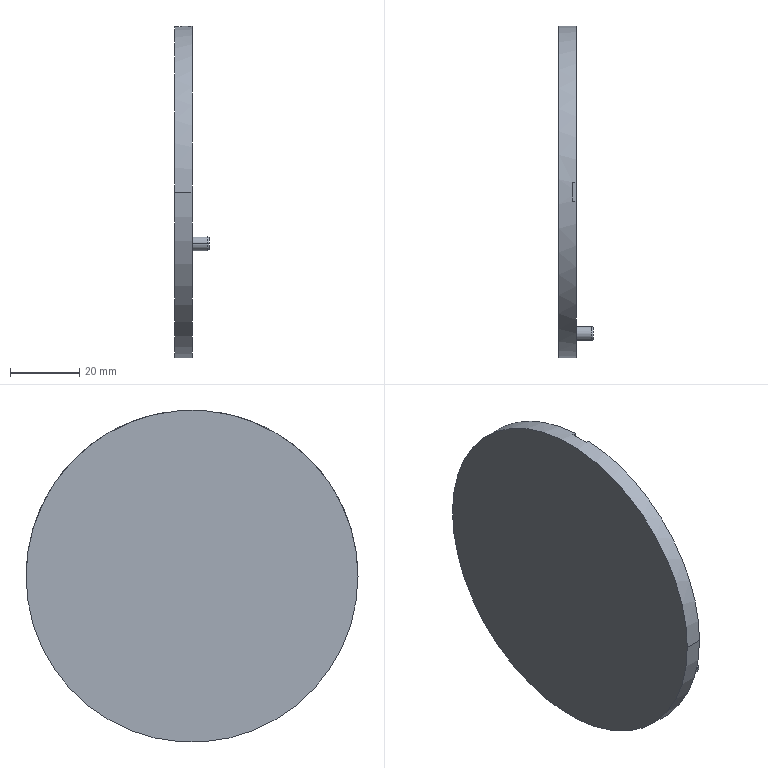Part | STEP file | ASND-0110-IRB120_3-58_IRC5_Link3_rev0 | 2 solids | 14 faces | box 10 x 96 x 96 mm | volume 36166 mm3 | plane 8 | cylinder 4 | cone 2 | commonest cylinder face diameters 4 x2 96 x2
STEP:
#1=CARTESIAN_POINT('',(0.,0.,0.));
#2=DIRECTION('',(0.,0.,1.));
#3=DIRECTION('',(1.,0.,0.));
#4=AXIS2_PLACEMENT_3D('',#1,#2,#3);
#5=CARTESIAN_POINT('',(144.6,48.,630.));
#6=VERTEX_POINT('',#5);
#7=CARTESIAN_POINT('',(144.6,-48.,630.));
#8=VERTEX_POINT('',#7);
#9=CARTESIAN_POINT('',(144.6,0.,630.));
#10=DIRECTION('',(-1.,0.,0.));
#11=DIRECTION('',(0.,1.,0.));
#12=AXIS2_PLACEMENT_3D('',#9,#10,#11);
#13=CIRCLE('',#12,48.);
#14=CARTESIAN_POINT('',(144.6,0.,630.));
#15=DIRECTION('',(1.,0.,0.));
#16=DIRECTION('',(0.,-1.,0.));
#17=AXIS2_PLACEMENT_3D('',#14,#15,#16);
#18=CYLINDRICAL_SURFACE('',#17,48.);
#19=CARTESIAN_POINT('',(3.142,0.));
#20=DIRECTION('',(-1.,0.));
#21=VECTOR('',#20,1.);
#22=LINE('',#19,#21);
#23=(GEOMETRIC_REPRESENTATION_CONTEXT(2)PARAMETRIC_REPRESENTATION_CONTEXT()REPRESENTATION_CONTEXT('',''));
#24=DEFINITIONAL_REPRESENTATION('',(#22),#23);
#25=PCURVE('',#18,#24);
#26=CARTESIAN_POINT('',(144.6,0.,630.));
#27=DIRECTION('',(-1.,0.,0.));
#28=DIRECTION('',(0.,0.7071,0.7071));
#29=AXIS2_PLACEMENT_3D('',#26,#27,#28);
#30=PLANE('',#29);
#31=CARTESIAN_POINT('',(0.,0.));
#32=DIRECTION('',(0.7071,0.7071));
#33=AXIS2_PLACEMENT_2D('',#31,#32);
#34=CIRCLE('',#33,48.);
#35=(GEOMETRIC_REPRESENTATION_CONTEXT(2)PARAMETRIC_REPRESENTATION_CONTEXT()REPRESENTATION_CONTEXT('',''));
#36=DEFINITIONAL_REPRESENTATION('',(#34),#35);
#37=PCURVE('',#30,#36);
#38=SURFACE_CURVE('',#13,(#25,#37),.PCURVE_S1.);
#39=EDGE_CURVE('',#6,#8,#38,.T.);
#40=ORIENTED_EDGE('',*,*,#39,.F.);
#41=CARTESIAN_POINT('',(149.6,48.,630.));
#42=VERTEX_POINT('',#41);
#43=CARTESIAN_POINT('',(144.6,48.,630.));
#44=DIRECTION('',(1.,0.,0.));
#45=VECTOR('',#44,1.);
#46=LINE('',#43,#45);
#47=CARTESIAN_POINT('',(3.142,0.));
#48=DIRECTION('',(0.,1.));
#49=VECTOR('',#48,1.);
#50=LINE('',#47,#49);
#51=(GEOMETRIC_REPRESENTATION_CONTEXT(2)PARAMETRIC_REPRESENTATION_CONTEXT()REPRESENTATION_CONTEXT('',''));
#52=DEFINITIONAL_REPRESENTATION('',(#50),#51);
#53=PCURVE('',#18,#52);
#54=CARTESIAN_POINT('',(144.6,0.,630.));
#55=DIRECTION('',(1.,0.,0.));
#56=DIRECTION('',(0.,-1.,0.));
#57=AXIS2_PLACEMENT_3D('',#54,#55,#56);
#58=CYLINDRICAL_SURFACE('',#57,48.);
#59=CARTESIAN_POINT('',(3.142,0.));
#60=DIRECTION('',(0.,1.));
#61=VECTOR('',#60,1.);
#62=LINE('',#59,#61);
#63=(GEOMETRIC_REPRESENTATION_CONTEXT(2)PARAMETRIC_REPRESENTATION_CONTEXT()REPRESENTATION_CONTEXT('',''));
#64=DEFINITIONAL_REPRESENTATION('',(#62),#63);
#65=PCURVE('',#58,#64);
#66=SURFACE_CURVE('',#46,(#53,#65),.PCURVE_S1.);
#67=EDGE_CURVE('',#6,#42,#66,.T.);
#68=ORIENTED_EDGE('',*,*,#67,.T.);
#69=CARTESIAN_POINT('',(149.6,-48.,630.));
#70=VERTEX_POINT('',#69);
#71=CARTESIAN_POINT('',(149.6,0.,630.));
#72=DIRECTION('',(-1.,0.,0.));
#73=DIRECTION('',(0.,1.,0.));
#74=AXIS2_PLACEMENT_3D('',#71,#72,#73);
#75=CIRCLE('',#74,48.);
#76=CARTESIAN_POINT('',(3.142,5.));
#77=DIRECTION('',(-1.,0.));
#78=VECTOR('',#77,1.);
#79=LINE('',#76,#78);
#80=(GEOMETRIC_REPRESENTATION_CONTEXT(2)PARAMETRIC_REPRESENTATION_CONTEXT()REPRESENTATION_CONTEXT('',''));
#81=DEFINITIONAL_REPRESENTATION('',(#79),#80);
#82=PCURVE('',#18,#81);
#83=CARTESIAN_POINT('',(149.6,0.,630.));
#84=DIRECTION('',(-1.,0.,0.));
#85=DIRECTION('',(0.,0.7071,0.7071));
#86=AXIS2_PLACEMENT_3D('',#83,#84,#85);
#87=PLANE('',#86);
#88=CARTESIAN_POINT('',(0.,0.));
#89=DIRECTION('',(0.7071,0.7071));
#90=AXIS2_PLACEMENT_2D('',#88,#89);
#91=CIRCLE('',#90,48.);
#92=(GEOMETRIC_REPRESENTATION_CONTEXT(2)PARAMETRIC_REPRESENTATION_CONTEXT()REPRESENTATION_CONTEXT('',''));
#93=DEFINITIONAL_REPRESENTATION('',(#91),#92);
#94=PCURVE('',#87,#93);
#95=SURFACE_CURVE('',#75,(#82,#94),.PCURVE_S1.);
#96=EDGE_CURVE('',#42,#70,#95,.T.);
#97=ORIENTED_EDGE('',*,*,#96,.T.);
#98=CARTESIAN_POINT('',(144.6,-48.,630.));
#99=DIRECTION('',(1.,0.,0.));
#100=VECTOR('',#99,1.);
#101=LINE('',#98,#100);
#102=CARTESIAN_POINT('',(0.,0.));
#103=DIRECTION('',(0.,1.));
#104=VECTOR('',#103,1.);
#105=LINE('',#102,#104);
#106=(GEOMETRIC_REPRESENTATION_CONTEXT(2)PARAMETRIC_REPRESENTATION_CONTEXT()REPRESENTATION_CONTEXT('',''));
#107=DEFINITIONAL_REPRESENTATION('',(#105),#106);
#108=PCURVE('',#18,#107);
#109=CARTESIAN_POINT('',(6.283,0.));
#110=DIRECTION('',(0.,1.));
#111=VECTOR('',#110,1.);
#112=LINE('',#109,#111);
#113=(GEOMETRIC_REPRESENTATION_CONTEXT(2)PARAMETRIC_REPRESENTATION_CONTEXT()REPRESENTATION_CONTEXT('',''));
#114=DEFINITIONAL_REPRESENTATION('',(#112),#113);
#115=PCURVE('',#58,#114);
#116=SURFACE_CURVE('',#101,(#108,#115),.PCURVE_S1.);
#117=EDGE_CURVE('',#8,#70,#116,.T.);
#118=ORIENTED_EDGE('',*,*,#117,.F.);
#119=EDGE_LOOP('',(#40,#68,#97,#118));
#120=FACE_BOUND('',#119,.T.);
#121=ADVANCED_FACE('',(#120),#18,.T.);
#122=ORIENTED_EDGE('',*,*,#67,.F.);
#123=CARTESIAN_POINT('',(144.6,0.,630.));
#124=DIRECTION('',(-1.,0.,0.));
#125=DIRECTION('',(0.,1.,0.));
#126=AXIS2_PLACEMENT_3D('',#123,#124,#125);
#127=CIRCLE('',#126,48.);
#128=CARTESIAN_POINT('',(9.425,0.));
#129=DIRECTION('',(-1.,0.));
#130=VECTOR('',#129,1.);
#131=LINE('',#128,#130);
#132=(GEOMETRIC_REPRESENTATION_CONTEXT(2)PARAMETRIC_REPRESENTATION_CONTEXT()REPRESENTATION_CONTEXT('',''));
#133=DEFINITIONAL_REPRESENTATION('',(#131),#132);
#134=PCURVE('',#58,#133);
#135=CARTESIAN_POINT('',(0.,0.));
#136=DIRECTION('',(0.7071,0.7071));
#137=AXIS2_PLACEMENT_2D('',#135,#136);
#138=CIRCLE('',#137,48.);
#139=(GEOMETRIC_REPRESENTATION_CONTEXT(2)PARAMETRIC_REPRESENTATION_CONTEXT()REPRESENTATION_CONTEXT('',''));
#140=DEFINITIONAL_REPRESENTATION('',(#138),#139);
#141=PCURVE('',#30,#140);
#142=SURFACE_CURVE('',#127,(#134,#141),.PCURVE_S1.);
#143=EDGE_CURVE('',#8,#6,#142,.T.);
#144=ORIENTED_EDGE('',*,*,#143,.F.);
#145=ORIENTED_EDGE('',*,*,#117,.T.);
#146=CARTESIAN_POINT('',(149.6,-2.75,677.921));
#147=VERTEX_POINT('',#146);
#148=CARTESIAN_POINT('',(149.6,0.,630.));
#149=DIRECTION('',(-1.,0.,0.));
#150=DIRECTION('',(0.,1.,0.));
#151=AXIS2_PLACEMENT_3D('',#148,#149,#150);
#152=CIRCLE('',#151,48.);
#153=CARTESIAN_POINT('',(9.425,5.));
#154=DIRECTION('',(-1.,0.));
#155=VECTOR('',#154,1.);
#156=LINE('',#153,#155);
#157=(GEOMETRIC_REPRESENTATION_CONTEXT(2)PARAMETRIC_REPRESENTATION_CONTEXT()REPRESENTATION_CONTEXT('',''));
#158=DEFINITIONAL_REPRESENTATION('',(#156),#157);
#159=PCURVE('',#58,#158);
#160=CARTESIAN_POINT('',(0.,0.));
#161=DIRECTION('',(0.7071,0.7071));
#162=AXIS2_PLACEMENT_2D('',#160,#161);
#163=CIRCLE('',#162,48.);
#164=(GEOMETRIC_REPRESENTATION_CONTEXT(2)PARAMETRIC_REPRESENTATION_CONTEXT()REPRESENTATION_CONTEXT('',''));
#165=DEFINITIONAL_REPRESENTATION('',(#163),#164);
#166=PCURVE('',#87,#165);
#167=SURFACE_CURVE('',#152,(#159,#166),.PCURVE_S1.);
#168=EDGE_CURVE('',#70,#147,#167,.T.);
#169=ORIENTED_EDGE('',*,*,#168,.T.);
#170=CARTESIAN_POINT('',(148.6,-2.75,677.921));
#171=VERTEX_POINT('',#170);
#172=CARTESIAN_POINT('',(148.6,-2.75,677.921));
#173=DIRECTION('',(-1.,0.,0.));
#174=VECTOR('',#173,1.);
#175=LINE('',#172,#174);
#176=CARTESIAN_POINT('',(4.77,4.));
#177=DIRECTION('',(0.,-1.));
#178=VECTOR('',#177,1.);
#179=LINE('',#176,#178);
#180=(GEOMETRIC_REPRESENTATION_CONTEXT(2)PARAMETRIC_REPRESENTATION_CONTEXT()REPRESENTATION_CONTEXT('',''));
#181=DEFINITIONAL_REPRESENTATION('',(#179),#180);
#182=PCURVE('',#58,#181);
#183=CARTESIAN_POINT('',(148.6,-2.75,662.));
#184=DIRECTION('',(0.,-1.,0.));
#185=DIRECTION('',(0.7071,0.,0.7071));
#186=AXIS2_PLACEMENT_3D('',#183,#184,#185);
#187=PLANE('',#186);
#188=CARTESIAN_POINT('',(11.258,11.258));
#189=DIRECTION('',(-0.7071,0.7071));
#190=VECTOR('',#189,1.);
#191=LINE('',#188,#190);
#192=(GEOMETRIC_REPRESENTATION_CONTEXT(2)PARAMETRIC_REPRESENTATION_CONTEXT()REPRESENTATION_CONTEXT('',''));
#193=DEFINITIONAL_REPRESENTATION('',(#191),#192);
#194=PCURVE('',#187,#193);
#195=SURFACE_CURVE('',#175,(#182,#194),.PCURVE_S1.);
#196=EDGE_CURVE('',#147,#171,#195,.T.);
#197=ORIENTED_EDGE('',*,*,#196,.T.);
#198=CARTESIAN_POINT('',(148.6,2.75,677.921));
#199=VERTEX_POINT('',#198);
#200=CARTESIAN_POINT('',(148.6,0.,630.));
#201=DIRECTION('',(1.,0.,0.));
#202=DIRECTION('',(0.,-1.,0.));
#203=AXIS2_PLACEMENT_3D('',#200,#201,#202);
#204=CIRCLE('',#203,48.);
#205=CARTESIAN_POINT('',(0.,4.));
#206=DIRECTION('',(1.,0.));
#207=VECTOR('',#206,1.);
#208=LINE('',#205,#207);
#209=(GEOMETRIC_REPRESENTATION_CONTEXT(2)PARAMETRIC_REPRESENTATION_CONTEXT()REPRESENTATION_CONTEXT('',''));
#210=DEFINITIONAL_REPRESENTATION('',(#208),#209);
#211=PCURVE('',#58,#210);
#212=CARTESIAN_POINT('',(148.6,2.75,682.));
#213=DIRECTION('',(1.,0.,0.));
#214=DIRECTION('',(0.,0.7071,0.7071));
#215=AXIS2_PLACEMENT_3D('',#212,#213,#214);
#216=PLANE('',#215);
#217=CARTESIAN_POINT('',(-38.714,-34.825));
#218=DIRECTION('',(-0.7071,0.7071));
#219=AXIS2_PLACEMENT_2D('',#217,#218);
#220=CIRCLE('',#219,48.);
#221=(GEOMETRIC_REPRESENTATION_CONTEXT(2)PARAMETRIC_REPRESENTATION_CONTEXT()REPRESENTATION_CONTEXT('',''));
#222=DEFINITIONAL_REPRESENTATION('',(#220),#221);
#223=PCURVE('',#216,#222);
#224=SURFACE_CURVE('',#204,(#211,#223),.PCURVE_S1.);
#225=EDGE_CURVE('',#199,#171,#224,.T.);
#226=ORIENTED_EDGE('',*,*,#225,.F.);
#227=CARTESIAN_POINT('',(149.6,2.75,677.921));
#228=VERTEX_POINT('',#227);
#229=CARTESIAN_POINT('',(148.6,2.75,677.921));
#230=DIRECTION('',(1.,0.,0.));
#231=VECTOR('',#230,1.);
#232=LINE('',#229,#231);
#233=CARTESIAN_POINT('',(4.655,4.));
#234=DIRECTION('',(0.,1.));
#235=VECTOR('',#234,1.);
#236=LINE('',#233,#235);
#237=(GEOMETRIC_REPRESENTATION_CONTEXT(2)PARAMETRIC_REPRESENTATION_CONTEXT()REPRESENTATION_CONTEXT('',''));
#238=DEFINITIONAL_REPRESENTATION('',(#236),#237);
#239=PCURVE('',#58,#238);
#240=CARTESIAN_POINT('',(148.6,2.75,662.));
#241=DIRECTION('',(0.,1.,0.));
#242=DIRECTION('',(0.7071,0.,0.7071));
#243=AXIS2_PLACEMENT_3D('',#240,#241,#242);
#244=PLANE('',#243);
#245=CARTESIAN_POINT('',(11.258,-11.258));
#246=DIRECTION('',(0.7071,0.7071));
#247=VECTOR('',#246,1.);
#248=LINE('',#245,#247);
#249=(GEOMETRIC_REPRESENTATION_CONTEXT(2)PARAMETRIC_REPRESENTATION_CONTEXT()REPRESENTATION_CONTEXT('',''));
#250=DEFINITIONAL_REPRESENTATION('',(#248),#249);
#251=PCURVE('',#244,#250);
#252=SURFACE_CURVE('',#232,(#239,#251),.PCURVE_S1.);
#253=EDGE_CURVE('',#199,#228,#252,.T.);
#254=ORIENTED_EDGE('',*,*,#253,.T.);
#255=CARTESIAN_POINT('',(149.6,0.,630.));
#256=DIRECTION('',(-1.,0.,0.));
#257=DIRECTION('',(0.,1.,0.));
#258=AXIS2_PLACEMENT_3D('',#255,#256,#257);
#259=CIRCLE('',#258,48.);
#260=CARTESIAN_POINT('',(9.425,5.));
#261=DIRECTION('',(-1.,0.));
#262=VECTOR('',#261,1.);
#263=LINE('',#260,#262);
#264=(GEOMETRIC_REPRESENTATION_CONTEXT(2)PARAMETRIC_REPRESENTATION_CONTEXT()REPRESENTATION_CONTEXT('',''));
#265=DEFINITIONAL_REPRESENTATION('',(#263),#264);
#266=PCURVE('',#58,#265);
#267=CARTESIAN_POINT('',(0.,0.));
#268=DIRECTION('',(0.7071,0.7071));
#269=AXIS2_PLACEMENT_2D('',#267,#268);
#270=CIRCLE('',#269,48.);
#271=(GEOMETRIC_REPRESENTATION_CONTEXT(2)PARAMETRIC_REPRESENTATION_CONTEXT()REPRESENTATION_CONTEXT('',''));
#272=DEFINITIONAL_REPRESENTATION('',(#270),#271);
#273=PCURVE('',#87,#272);
#274=SURFACE_CURVE('',#259,(#266,#273),.PCURVE_S1.);
#275=EDGE_CURVE('',#228,#42,#274,.T.);
#276=ORIENTED_EDGE('',*,*,#275,.T.);
#277=EDGE_LOOP('',(#122,#144,#145,#169,#197,#226,#254,#276));
#278=FACE_BOUND('',#277,.T.);
#279=ADVANCED_FACE('',(#278),#58,.T.);
#280=ORIENTED_EDGE('',*,*,#143,.T.);
#281=ORIENTED_EDGE('',*,*,#39,.T.);
#282=EDGE_LOOP('',(#280,#281));
#283=FACE_BOUND('',#282,.T.);
#284=ADVANCED_FACE('',(#283),#30,.T.);
#285=ORIENTED_EDGE('',*,*,#275,.F.);
#286=CARTESIAN_POINT('',(149.6,2.75,662.));
#287=VERTEX_POINT('',#286);
#288=CARTESIAN_POINT('',(149.6,2.75,662.));
#289=DIRECTION('',(0.,0.,1.));
#290=VECTOR('',#289,1.);
#291=LINE('',#288,#290);
#292=CARTESIAN_POINT('',(24.572,-20.683));
#293=DIRECTION('',(0.7071,-0.7071));
#294=VECTOR('',#293,1.);
#295=LINE('',#292,#294);
#296=(GEOMETRIC_REPRESENTATION_CONTEXT(2)PARAMETRIC_REPRESENTATION_CONTEXT()REPRESENTATION_CONTEXT('',''));
#297=DEFINITIONAL_REPRESENTATION('',(#295),#296);
#298=PCURVE('',#87,#297);
#299=CARTESIAN_POINT('',(0.7071,0.7071));
#300=DIRECTION('',(0.7071,-0.7071));
#301=VECTOR('',#300,1.);
#302=LINE('',#299,#301);
#303=(GEOMETRIC_REPRESENTATION_CONTEXT(2)PARAMETRIC_REPRESENTATION_CONTEXT()REPRESENTATION_CONTEXT('',''));
#304=DEFINITIONAL_REPRESENTATION('',(#302),#303);
#305=PCURVE('',#244,#304);
#306=SURFACE_CURVE('',#291,(#298,#305),.PCURVE_S1.);
#307=EDGE_CURVE('',#287,#228,#306,.T.);
#308=ORIENTED_EDGE('',*,*,#307,.F.);
#309=CARTESIAN_POINT('',(149.6,-2.75,662.));
#310=VERTEX_POINT('',#309);
#311=CARTESIAN_POINT('',(149.6,-2.75,662.));
#312=DIRECTION('',(0.,1.,0.));
#313=VECTOR('',#312,1.);
#314=LINE('',#311,#313);
#315=CARTESIAN_POINT('',(20.683,-24.572));
#316=DIRECTION('',(0.7071,0.7071));
#317=VECTOR('',#316,1.);
#318=LINE('',#315,#317);
#319=(GEOMETRIC_REPRESENTATION_CONTEXT(2)PARAMETRIC_REPRESENTATION_CONTEXT()REPRESENTATION_CONTEXT('',''));
#320=DEFINITIONAL_REPRESENTATION('',(#318),#319);
#321=PCURVE('',#87,#320);
#322=CARTESIAN_POINT('',(148.6,2.75,662.));
#323=DIRECTION('',(0.,0.,-1.));
#324=DIRECTION('',(0.7071,0.7071,0.));
#325=AXIS2_PLACEMENT_3D('',#322,#323,#324);
#326=PLANE('',#325);
#327=CARTESIAN_POINT('',(-3.182,4.596));
#328=DIRECTION('',(0.7071,-0.7071));
#329=VECTOR('',#328,1.);
#330=LINE('',#327,#329);
#331=(GEOMETRIC_REPRESENTATION_CONTEXT(2)PARAMETRIC_REPRESENTATION_CONTEXT()REPRESENTATION_CONTEXT('',''));
#332=DEFINITIONAL_REPRESENTATION('',(#330),#331);
#333=PCURVE('',#326,#332);
#334=SURFACE_CURVE('',#314,(#321,#333),.PCURVE_S1.);
#335=EDGE_CURVE('',#310,#287,#334,.T.);
#336=ORIENTED_EDGE('',*,*,#335,.F.);
#337=CARTESIAN_POINT('',(149.6,-2.75,662.));
#338=DIRECTION('',(0.,0.,1.));
#339=VECTOR('',#338,1.);
#340=LINE('',#337,#339);
#341=CARTESIAN_POINT('',(20.683,-24.572));
#342=DIRECTION('',(0.7071,-0.7071));
#343=VECTOR('',#342,1.);
#344=LINE('',#341,#343);
#345=(GEOMETRIC_REPRESENTATION_CONTEXT(2)PARAMETRIC_REPRESENTATION_CONTEXT()REPRESENTATION_CONTEXT('',''));
#346=DEFINITIONAL_REPRESENTATION('',(#344),#345);
#347=PCURVE('',#87,#346);
#348=CARTESIAN_POINT('',(0.7071,-0.7071));
#349=DIRECTION('',(0.7071,0.7071));
#350=VECTOR('',#349,1.);
#351=LINE('',#348,#350);
#352=(GEOMETRIC_REPRESENTATION_CONTEXT(2)PARAMETRIC_REPRESENTATION_CONTEXT()REPRESENTATION_CONTEXT('',''));
#353=DEFINITIONAL_REPRESENTATION('',(#351),#352);
#354=PCURVE('',#187,#353);
#355=SURFACE_CURVE('',#340,(#347,#354),.PCURVE_S1.);
#356=EDGE_CURVE('',#310,#147,#355,.T.);
#357=ORIENTED_EDGE('',*,*,#356,.T.);
#358=ORIENTED_EDGE('',*,*,#168,.F.);
#359=ORIENTED_EDGE('',*,*,#96,.F.);
#360=EDGE_LOOP('',(#285,#308,#336,#357,#358,#359));
#361=FACE_BOUND('',#360,.T.);
#362=ADVANCED_FACE('',(#361),#87,.F.);
#363=ORIENTED_EDGE('',*,*,#225,.T.);
#364=CARTESIAN_POINT('',(148.6,-2.75,662.));
#365=VERTEX_POINT('',#364);
#366=CARTESIAN_POINT('',(148.6,-2.75,677.921));
#367=DIRECTION('',(0.,0.,-1.));
#368=VECTOR('',#367,1.);
#369=LINE('',#366,#368);
#370=CARTESIAN_POINT('',(-6.773,1.005));
#371=DIRECTION('',(-0.7071,-0.7071));
#372=VECTOR('',#371,1.);
#373=LINE('',#370,#372);
#374=(GEOMETRIC_REPRESENTATION_CONTEXT(2)PARAMETRIC_REPRESENTATION_CONTEXT()REPRESENTATION_CONTEXT('',''));
#375=DEFINITIONAL_REPRESENTATION('',(#373),#374);
#376=PCURVE('',#216,#375);
#377=CARTESIAN_POINT('',(11.258,11.258));
#378=DIRECTION('',(-0.7071,-0.7071));
#379=VECTOR('',#378,1.);
#380=LINE('',#377,#379);
#381=(GEOMETRIC_REPRESENTATION_CONTEXT(2)PARAMETRIC_REPRESENTATION_CONTEXT()REPRESENTATION_CONTEXT('',''));
#382=DEFINITIONAL_REPRESENTATION('',(#380),#381);
#383=PCURVE('',#187,#382);
#384=SURFACE_CURVE('',#369,(#376,#383),.PCURVE_S1.);
#385=EDGE_CURVE('',#171,#365,#384,.T.);
#386=ORIENTED_EDGE('',*,*,#385,.T.);
#387=CARTESIAN_POINT('',(148.6,2.75,662.));
#388=VERTEX_POINT('',#387);
#389=CARTESIAN_POINT('',(148.6,-2.75,662.));
#390=DIRECTION('',(0.,1.,0.));
#391=VECTOR('',#390,1.);
#392=LINE('',#389,#391);
#393=CARTESIAN_POINT('',(-18.031,-10.253));
#394=DIRECTION('',(0.7071,-0.7071));
#395=VECTOR('',#394,1.);
#396=LINE('',#393,#395);
#397=(GEOMETRIC_REPRESENTATION_CONTEXT(2)PARAMETRIC_REPRESENTATION_CONTEXT()REPRESENTATION_CONTEXT('',''));
#398=DEFINITIONAL_REPRESENTATION('',(#396),#397);
#399=PCURVE('',#216,#398);
#400=CARTESIAN_POINT('',(-3.889,3.889));
#401=DIRECTION('',(0.7071,-0.7071));
#402=VECTOR('',#401,1.);
#403=LINE('',#400,#402);
#404=(GEOMETRIC_REPRESENTATION_CONTEXT(2)PARAMETRIC_REPRESENTATION_CONTEXT()REPRESENTATION_CONTEXT('',''));
#405=DEFINITIONAL_REPRESENTATION('',(#403),#404);
#406=PCURVE('',#326,#405);
#407=SURFACE_CURVE('',#392,(#399,#406),.PCURVE_S1.);
#408=EDGE_CURVE('',#365,#388,#407,.T.);
#409=ORIENTED_EDGE('',*,*,#408,.T.);
#410=CARTESIAN_POINT('',(148.6,2.75,662.));
#411=DIRECTION('',(0.,0.,1.));
#412=VECTOR('',#411,1.);
#413=LINE('',#410,#412);
#414=CARTESIAN_POINT('',(-14.142,-14.142));
#415=DIRECTION('',(0.7071,0.7071));
#416=VECTOR('',#415,1.);
#417=LINE('',#414,#416);
#418=(GEOMETRIC_REPRESENTATION_CONTEXT(2)PARAMETRIC_REPRESENTATION_CONTEXT()REPRESENTATION_CONTEXT('',''));
#419=DEFINITIONAL_REPRESENTATION('',(#417),#418);
#420=PCURVE('',#216,#419);
#421=CARTESIAN_POINT('',(0.,0.));
#422=DIRECTION('',(0.7071,-0.7071));
#423=VECTOR('',#422,1.);
#424=LINE('',#421,#423);
#425=(GEOMETRIC_REPRESENTATION_CONTEXT(2)PARAMETRIC_REPRESENTATION_CONTEXT()REPRESENTATION_CONTEXT('',''));
#426=DEFINITIONAL_REPRESENTATION('',(#424),#425);
#427=PCURVE('',#244,#426);
#428=SURFACE_CURVE('',#413,(#420,#427),.PCURVE_S1.);
#429=EDGE_CURVE('',#388,#199,#428,.T.);
#430=ORIENTED_EDGE('',*,*,#429,.T.);
#431=EDGE_LOOP('',(#363,#386,#409,#430));
#432=FACE_BOUND('',#431,.T.);
#433=ADVANCED_FACE('',(#432),#216,.T.);
#434=ORIENTED_EDGE('',*,*,#429,.F.);
#435=CARTESIAN_POINT('',(148.6,2.75,662.));
#436=DIRECTION('',(1.,0.,0.));
#437=VECTOR('',#436,1.);
#438=LINE('',#435,#437);
#439=CARTESIAN_POINT('',(0.,0.));
#440=DIRECTION('',(0.7071,0.7071));
#441=VECTOR('',#440,1.);
#442=LINE('',#439,#441);
#443=(GEOMETRIC_REPRESENTATION_CONTEXT(2)PARAMETRIC_REPRESENTATION_CONTEXT()REPRESENTATION_CONTEXT('',''));
#444=DEFINITIONAL_REPRESENTATION('',(#442),#443);
#445=PCURVE('',#244,#444);
#446=CARTESIAN_POINT('',(0.,0.));
#447=DIRECTION('',(0.7071,0.7071));
#448=VECTOR('',#447,1.);
#449=LINE('',#446,#448);
#450=(GEOMETRIC_REPRESENTATION_CONTEXT(2)PARAMETRIC_REPRESENTATION_CONTEXT()REPRESENTATION_CONTEXT('',''));
#451=DEFINITIONAL_REPRESENTATION('',(#449),#450);
#452=PCURVE('',#326,#451);
#453=SURFACE_CURVE('',#438,(#445,#452),.PCURVE_S1.);
#454=EDGE_CURVE('',#388,#287,#453,.T.);
#455=ORIENTED_EDGE('',*,*,#454,.T.);
#456=ORIENTED_EDGE('',*,*,#307,.T.);
#457=ORIENTED_EDGE('',*,*,#253,.F.);
#458=EDGE_LOOP('',(#434,#455,#456,#457));
#459=FACE_BOUND('',#458,.T.);
#460=ADVANCED_FACE('',(#459),#244,.F.);
#461=ORIENTED_EDGE('',*,*,#356,.F.);
#462=CARTESIAN_POINT('',(148.6,-2.75,662.));
#463=DIRECTION('',(1.,0.,0.));
#464=VECTOR('',#463,1.);
#465=LINE('',#462,#464);
#466=CARTESIAN_POINT('',(0.,0.));
#467=DIRECTION('',(0.7071,-0.7071));
#468=VECTOR('',#467,1.);
#469=LINE('',#466,#468);
#470=(GEOMETRIC_REPRESENTATION_CONTEXT(2)PARAMETRIC_REPRESENTATION_CONTEXT()REPRESENTATION_CONTEXT('',''));
#471=DEFINITIONAL_REPRESENTATION('',(#469),#470);
#472=PCURVE('',#187,#471);
#473=CARTESIAN_POINT('',(-3.889,3.889));
#474=DIRECTION('',(0.7071,0.7071));
#475=VECTOR('',#474,1.);
#476=LINE('',#473,#475);
#477=(GEOMETRIC_REPRESENTATION_CONTEXT(2)PARAMETRIC_REPRESENTATION_CONTEXT()REPRESENTATION_CONTEXT('',''));
#478=DEFINITIONAL_REPRESENTATION('',(#476),#477);
#479=PCURVE('',#326,#478);
#480=SURFACE_CURVE('',#465,(#472,#479),.PCURVE_S1.);
#481=EDGE_CURVE('',#365,#310,#480,.T.);
#482=ORIENTED_EDGE('',*,*,#481,.F.);
#483=ORIENTED_EDGE('',*,*,#385,.F.);
#484=ORIENTED_EDGE('',*,*,#196,.F.);
#485=EDGE_LOOP('',(#461,#482,#483,#484));
#486=FACE_BOUND('',#485,.T.);
#487=ADVANCED_FACE('',(#486),#187,.F.);
#488=ORIENTED_EDGE('',*,*,#335,.T.);
#489=ORIENTED_EDGE('',*,*,#454,.F.);
#490=ORIENTED_EDGE('',*,*,#408,.F.);
#491=ORIENTED_EDGE('',*,*,#481,.T.);
#492=EDGE_LOOP('',(#488,#489,#490,#491));
#493=FACE_BOUND('',#492,.T.);
#494=ADVANCED_FACE('',(#493),#326,.F.);
#495=CLOSED_SHELL('',(#121,#279,#284,#362,#433,#460,#487,#494));
#496=MANIFOLD_SOLID_BREP('',#495);
#497=CARTESIAN_POINT('',(154.6,-42.716,615.122));
#498=VERTEX_POINT('',#497);
#499=CARTESIAN_POINT('',(154.6,-39.037,615.122));
#500=VERTEX_POINT('',#499);
#501=CARTESIAN_POINT('',(154.6,-40.877,615.122));
#502=DIRECTION('',(-1.,0.,0.));
#503=DIRECTION('',(0.,-1.,0.));
#504=AXIS2_PLACEMENT_3D('',#501,#502,#503);
#505=CIRCLE('',#504,1.839);
#506=CARTESIAN_POINT('',(154.6,-40.877,615.122));
#507=DIRECTION('',(-1.,0.,0.));
#508=DIRECTION('',(0.,-1.,0.));
#509=AXIS2_PLACEMENT_3D('',#506,#507,#508);
#510=CONICAL_SURFACE('',#509,1.839,0.2618);
#511=CARTESIAN_POINT('',(0.,0.));
#512=DIRECTION('',(1.,0.));
#513=VECTOR('',#512,1.);
#514=LINE('',#511,#513);
#515=(GEOMETRIC_REPRESENTATION_CONTEXT(2)PARAMETRIC_REPRESENTATION_CONTEXT()REPRESENTATION_CONTEXT('',''));
#516=DEFINITIONAL_REPRESENTATION('',(#514),#515);
#517=PCURVE('',#510,#516);
#518=CARTESIAN_POINT('',(154.6,-39.037,615.122));
#519=DIRECTION('',(-1.,0.,0.));
#520=DIRECTION('',(0.,0.7071,0.7071));
#521=AXIS2_PLACEMENT_3D('',#518,#519,#520);
#522=PLANE('',#521);
#523=CARTESIAN_POINT('',(-1.301,-1.301));
#524=DIRECTION('',(-0.7071,-0.7071));
#525=AXIS2_PLACEMENT_2D('',#523,#524);
#526=CIRCLE('',#525,1.839);
#527=(GEOMETRIC_REPRESENTATION_CONTEXT(2)PARAMETRIC_REPRESENTATION_CONTEXT()REPRESENTATION_CONTEXT('',''));
#528=DEFINITIONAL_REPRESENTATION('',(#526),#527);
#529=PCURVE('',#522,#528);
#530=SURFACE_CURVE('',#505,(#517,#529),.PCURVE_S1.);
#531=EDGE_CURVE('',#498,#500,#530,.T.);
#532=ORIENTED_EDGE('',*,*,#531,.T.);
#533=CARTESIAN_POINT('',(154.,-38.877,615.122));
#534=VERTEX_POINT('',#533);
#535=CARTESIAN_POINT('',(154.6,-39.037,615.122));
#536=DIRECTION('',(-0.9659,0.2588,0.));
#537=VECTOR('',#536,1.);
#538=LINE('',#535,#537);
#539=CARTESIAN_POINT('',(3.142,0.));
#540=DIRECTION('',(0.,1.));
#541=VECTOR('',#540,1.);
#542=LINE('',#539,#541);
#543=(GEOMETRIC_REPRESENTATION_CONTEXT(2)PARAMETRIC_REPRESENTATION_CONTEXT()REPRESENTATION_CONTEXT('',''));
#544=DEFINITIONAL_REPRESENTATION('',(#542),#543);
#545=PCURVE('',#510,#544);
#546=CARTESIAN_POINT('',(154.6,-40.877,615.122));
#547=DIRECTION('',(-1.,0.,0.));
#548=DIRECTION('',(0.,-1.,0.));
#549=AXIS2_PLACEMENT_3D('',#546,#547,#548);
#550=CONICAL_SURFACE('',#549,1.839,0.2618);
#551=CARTESIAN_POINT('',(3.142,0.));
#552=DIRECTION('',(0.,1.));
#553=VECTOR('',#552,1.);
#554=LINE('',#551,#553);
#555=(GEOMETRIC_REPRESENTATION_CONTEXT(2)PARAMETRIC_REPRESENTATION_CONTEXT()REPRESENTATION_CONTEXT('',''));
#556=DEFINITIONAL_REPRESENTATION('',(#554),#555);
#557=PCURVE('',#550,#556);
#558=SURFACE_CURVE('',#538,(#545,#557),.PCURVE_S1.);
#559=EDGE_CURVE('',#500,#534,#558,.T.);
#560=ORIENTED_EDGE('',*,*,#559,.T.);
#561=CARTESIAN_POINT('',(154.,-42.877,615.122));
#562=VERTEX_POINT('',#561);
#563=CARTESIAN_POINT('',(154.,-40.877,615.122));
#564=DIRECTION('',(-1.,0.,0.));
#565=DIRECTION('',(0.,-1.,0.));
#566=AXIS2_PLACEMENT_3D('',#563,#564,#565);
#567=CIRCLE('',#566,2.);
#568=CARTESIAN_POINT('',(0.,0.6));
#569=DIRECTION('',(1.,0.));
#570=VECTOR('',#569,1.);
#571=LINE('',#568,#570);
#572=(GEOMETRIC_REPRESENTATION_CONTEXT(2)PARAMETRIC_REPRESENTATION_CONTEXT()REPRESENTATION_CONTEXT('',''));
#573=DEFINITIONAL_REPRESENTATION('',(#571),#572);
#574=PCURVE('',#510,#573);
#575=CARTESIAN_POINT('',(136.161,-40.877,615.122));
#576=DIRECTION('',(-1.,0.,0.));
#577=DIRECTION('',(0.,-1.,0.));
#578=AXIS2_PLACEMENT_3D('',#575,#576,#577);
#579=CYLINDRICAL_SURFACE('',#578,2.);
#580=CARTESIAN_POINT('',(0.,-17.839));
#581=DIRECTION('',(1.,0.));
#582=VECTOR('',#581,1.);
#583=LINE('',#580,#582);
#584=(GEOMETRIC_REPRESENTATION_CONTEXT(2)PARAMETRIC_REPRESENTATION_CONTEXT()REPRESENTATION_CONTEXT('',''));
#585=DEFINITIONAL_REPRESENTATION('',(#583),#584);
#586=PCURVE('',#579,#585);
#587=SURFACE_CURVE('',#567,(#574,#586),.PCURVE_S1.);
#588=EDGE_CURVE('',#562,#534,#587,.T.);
#589=ORIENTED_EDGE('',*,*,#588,.F.);
#590=CARTESIAN_POINT('',(154.6,-42.716,615.122));
#591=DIRECTION('',(-0.9659,-0.2588,0.));
#592=VECTOR('',#591,1.);
#593=LINE('',#590,#592);
#594=CARTESIAN_POINT('',(0.,0.));
#595=DIRECTION('',(0.,1.));
#596=VECTOR('',#595,1.);
#597=LINE('',#594,#596);
#598=(GEOMETRIC_REPRESENTATION_CONTEXT(2)PARAMETRIC_REPRESENTATION_CONTEXT()REPRESENTATION_CONTEXT('',''));
#599=DEFINITIONAL_REPRESENTATION('',(#597),#598);
#600=PCURVE('',#510,#599);
#601=CARTESIAN_POINT('',(6.283,0.));
#602=DIRECTION('',(0.,1.));
#603=VECTOR('',#602,1.);
#604=LINE('',#601,#603);
#605=(GEOMETRIC_REPRESENTATION_CONTEXT(2)PARAMETRIC_REPRESENTATION_CONTEXT()REPRESENTATION_CONTEXT('',''));
#606=DEFINITIONAL_REPRESENTATION('',(#604),#605);
#607=PCURVE('',#550,#606);
#608=SURFACE_CURVE('',#593,(#600,#607),.PCURVE_S1.);
#609=EDGE_CURVE('',#498,#562,#608,.T.);
#610=ORIENTED_EDGE('',*,*,#609,.F.);
#611=EDGE_LOOP('',(#532,#560,#589,#610));
#612=FACE_BOUND('',#611,.T.);
#613=ADVANCED_FACE('',(#612),#510,.T.);
#614=ORIENTED_EDGE('',*,*,#588,.T.);
#615=CARTESIAN_POINT('',(149.6,-38.877,615.122));
#616=VERTEX_POINT('',#615);
#617=CARTESIAN_POINT('',(136.161,-38.877,615.122));
#618=DIRECTION('',(-1.,0.,0.));
#619=VECTOR('',#618,1.);
#620=LINE('',#617,#619);
#621=CARTESIAN_POINT('',(3.142,0.));
#622=DIRECTION('',(0.,1.));
#623=VECTOR('',#622,1.);
#624=LINE('',#621,#623);
#625=(GEOMETRIC_REPRESENTATION_CONTEXT(2)PARAMETRIC_REPRESENTATION_CONTEXT()REPRESENTATION_CONTEXT('',''));
#626=DEFINITIONAL_REPRESENTATION('',(#624),#625);
#627=PCURVE('',#579,#626);
#628=CARTESIAN_POINT('',(136.161,-40.877,615.122));
#629=DIRECTION('',(-1.,0.,0.));
#630=DIRECTION('',(0.,-1.,0.));
#631=AXIS2_PLACEMENT_3D('',#628,#629,#630);
#632=CYLINDRICAL_SURFACE('',#631,2.);
#633=CARTESIAN_POINT('',(3.142,0.));
#634=DIRECTION('',(0.,1.));
#635=VECTOR('',#634,1.);
#636=LINE('',#633,#635);
#637=(GEOMETRIC_REPRESENTATION_CONTEXT(2)PARAMETRIC_REPRESENTATION_CONTEXT()REPRESENTATION_CONTEXT('',''));
#638=DEFINITIONAL_REPRESENTATION('',(#636),#637);
#639=PCURVE('',#632,#638);
#640=SURFACE_CURVE('',#620,(#627,#639),.PCURVE_S1.);
#641=EDGE_CURVE('',#534,#616,#640,.T.);
#642=ORIENTED_EDGE('',*,*,#641,.T.);
#643=CARTESIAN_POINT('',(149.6,-42.877,615.122));
#644=VERTEX_POINT('',#643);
#645=CARTESIAN_POINT('',(149.6,-40.877,615.122));
#646=DIRECTION('',(-1.,0.,0.));
#647=DIRECTION('',(0.,-1.,0.));
#648=AXIS2_PLACEMENT_3D('',#645,#646,#647);
#649=CIRCLE('',#648,2.);
#650=CARTESIAN_POINT('',(0.,-13.439));
#651=DIRECTION('',(1.,0.));
#652=VECTOR('',#651,1.);
#653=LINE('',#650,#652);
#654=(GEOMETRIC_REPRESENTATION_CONTEXT(2)PARAMETRIC_REPRESENTATION_CONTEXT()REPRESENTATION_CONTEXT('',''));
#655=DEFINITIONAL_REPRESENTATION('',(#653),#654);
#656=PCURVE('',#579,#655);
#657=CARTESIAN_POINT('',(149.6,-40.877,615.122));
#658=DIRECTION('',(-1.,0.,0.));
#659=DIRECTION('',(0.,0.7071,0.7071));
#660=AXIS2_PLACEMENT_3D('',#657,#658,#659);
#661=PLANE('',#660);
#662=CARTESIAN_POINT('',(0.,0.));
#663=DIRECTION('',(-0.7071,-0.7071));
#664=AXIS2_PLACEMENT_2D('',#662,#663);
#665=CIRCLE('',#664,2.);
#666=(GEOMETRIC_REPRESENTATION_CONTEXT(2)PARAMETRIC_REPRESENTATION_CONTEXT()REPRESENTATION_CONTEXT('',''));
#667=DEFINITIONAL_REPRESENTATION('',(#665),#666);
#668=PCURVE('',#661,#667);
#669=SURFACE_CURVE('',#649,(#656,#668),.PCURVE_S1.);
#670=EDGE_CURVE('',#644,#616,#669,.T.);
#671=ORIENTED_EDGE('',*,*,#670,.F.);
#672=CARTESIAN_POINT('',(136.161,-42.877,615.122));
#673=DIRECTION('',(-1.,0.,0.));
#674=VECTOR('',#673,1.);
#675=LINE('',#672,#674);
#676=CARTESIAN_POINT('',(0.,0.));
#677=DIRECTION('',(0.,1.));
#678=VECTOR('',#677,1.);
#679=LINE('',#676,#678);
#680=(GEOMETRIC_REPRESENTATION_CONTEXT(2)PARAMETRIC_REPRESENTATION_CONTEXT()REPRESENTATION_CONTEXT('',''));
#681=DEFINITIONAL_REPRESENTATION('',(#679),#680);
#682=PCURVE('',#579,#681);
#683=CARTESIAN_POINT('',(6.283,0.));
#684=DIRECTION('',(0.,1.));
#685=VECTOR('',#684,1.);
#686=LINE('',#683,#685);
#687=(GEOMETRIC_REPRESENTATION_CONTEXT(2)PARAMETRIC_REPRESENTATION_CONTEXT()REPRESENTATION_CONTEXT('',''));
#688=DEFINITIONAL_REPRESENTATION('',(#686),#687);
#689=PCURVE('',#632,#688);
#690=SURFACE_CURVE('',#675,(#682,#689),.PCURVE_S1.);
#691=EDGE_CURVE('',#562,#644,#690,.T.);
#692=ORIENTED_EDGE('',*,*,#691,.F.);
#693=EDGE_LOOP('',(#614,#642,#671,#692));
#694=FACE_BOUND('',#693,.T.);
#695=ADVANCED_FACE('',(#694),#579,.T.);
#696=ORIENTED_EDGE('',*,*,#641,.F.);
#697=CARTESIAN_POINT('',(154.,-40.877,615.122));
#698=DIRECTION('',(-1.,0.,0.));
#699=DIRECTION('',(0.,-1.,0.));
#700=AXIS2_PLACEMENT_3D('',#697,#698,#699);
#701=CIRCLE('',#700,2.);
#702=CARTESIAN_POINT('',(0.,-17.839));
#703=DIRECTION('',(1.,0.));
#704=VECTOR('',#703,1.);
#705=LINE('',#702,#704);
#706=(GEOMETRIC_REPRESENTATION_CONTEXT(2)PARAMETRIC_REPRESENTATION_CONTEXT()REPRESENTATION_CONTEXT('',''));
#707=DEFINITIONAL_REPRESENTATION('',(#705),#706);
#708=PCURVE('',#632,#707);
#709=CARTESIAN_POINT('',(0.,0.6));
#710=DIRECTION('',(1.,0.));
#711=VECTOR('',#710,1.);
#712=LINE('',#709,#711);
#713=(GEOMETRIC_REPRESENTATION_CONTEXT(2)PARAMETRIC_REPRESENTATION_CONTEXT()REPRESENTATION_CONTEXT('',''));
#714=DEFINITIONAL_REPRESENTATION('',(#712),#713);
#715=PCURVE('',#550,#714);
#716=SURFACE_CURVE('',#701,(#708,#715),.PCURVE_S1.);
#717=EDGE_CURVE('',#534,#562,#716,.T.);
#718=ORIENTED_EDGE('',*,*,#717,.T.);
#719=ORIENTED_EDGE('',*,*,#691,.T.);
#720=CARTESIAN_POINT('',(149.6,-40.877,615.122));
#721=DIRECTION('',(-1.,0.,0.));
#722=DIRECTION('',(0.,-1.,0.));
#723=AXIS2_PLACEMENT_3D('',#720,#721,#722);
#724=CIRCLE('',#723,2.);
#725=CARTESIAN_POINT('',(0.,-13.439));
#726=DIRECTION('',(1.,0.));
#727=VECTOR('',#726,1.);
#728=LINE('',#725,#727);
#729=(GEOMETRIC_REPRESENTATION_CONTEXT(2)PARAMETRIC_REPRESENTATION_CONTEXT()REPRESENTATION_CONTEXT('',''));
#730=DEFINITIONAL_REPRESENTATION('',(#728),#729);
#731=PCURVE('',#632,#730);
#732=CARTESIAN_POINT('',(0.,0.));
#733=DIRECTION('',(-0.7071,-0.7071));
#734=AXIS2_PLACEMENT_2D('',#732,#733);
#735=CIRCLE('',#734,2.);
#736=(GEOMETRIC_REPRESENTATION_CONTEXT(2)PARAMETRIC_REPRESENTATION_CONTEXT()REPRESENTATION_CONTEXT('',''));
#737=DEFINITIONAL_REPRESENTATION('',(#735),#736);
#738=PCURVE('',#661,#737);
#739=SURFACE_CURVE('',#724,(#731,#738),.PCURVE_S1.);
#740=EDGE_CURVE('',#616,#644,#739,.T.);
#741=ORIENTED_EDGE('',*,*,#740,.F.);
#742=EDGE_LOOP('',(#696,#718,#719,#741));
#743=FACE_BOUND('',#742,.T.);
#744=ADVANCED_FACE('',(#743),#632,.T.);
#745=ORIENTED_EDGE('',*,*,#559,.F.);
#746=CARTESIAN_POINT('',(154.6,-40.877,615.122));
#747=DIRECTION('',(-1.,0.,0.));
#748=DIRECTION('',(0.,-1.,0.));
#749=AXIS2_PLACEMENT_3D('',#746,#747,#748);
#750=CIRCLE('',#749,1.839);
#751=CARTESIAN_POINT('',(0.,0.));
#752=DIRECTION('',(1.,0.));
#753=VECTOR('',#752,1.);
#754=LINE('',#751,#753);
#755=(GEOMETRIC_REPRESENTATION_CONTEXT(2)PARAMETRIC_REPRESENTATION_CONTEXT()REPRESENTATION_CONTEXT('',''));
#756=DEFINITIONAL_REPRESENTATION('',(#754),#755);
#757=PCURVE('',#550,#756);
#758=CARTESIAN_POINT('',(-1.301,-1.301));
#759=DIRECTION('',(-0.7071,-0.7071));
#760=AXIS2_PLACEMENT_2D('',#758,#759);
#761=CIRCLE('',#760,1.839);
#762=(GEOMETRIC_REPRESENTATION_CONTEXT(2)PARAMETRIC_REPRESENTATION_CONTEXT()REPRESENTATION_CONTEXT('',''));
#763=DEFINITIONAL_REPRESENTATION('',(#761),#762);
#764=PCURVE('',#522,#763);
#765=SURFACE_CURVE('',#750,(#757,#764),.PCURVE_S1.);
#766=EDGE_CURVE('',#500,#498,#765,.T.);
#767=ORIENTED_EDGE('',*,*,#766,.T.);
#768=ORIENTED_EDGE('',*,*,#609,.T.);
#769=ORIENTED_EDGE('',*,*,#717,.F.);
#770=EDGE_LOOP('',(#745,#767,#768,#769));
#771=FACE_BOUND('',#770,.T.);
#772=ADVANCED_FACE('',(#771),#550,.T.);
#773=ORIENTED_EDGE('',*,*,#531,.F.);
#774=ORIENTED_EDGE('',*,*,#766,.F.);
#775=EDGE_LOOP('',(#773,#774));
#776=FACE_BOUND('',#775,.T.);
#777=ADVANCED_FACE('',(#776),#522,.F.);
#778=ORIENTED_EDGE('',*,*,#670,.T.);
#779=ORIENTED_EDGE('',*,*,#740,.T.);
#780=EDGE_LOOP('',(#778,#779));
#781=FACE_BOUND('',#780,.T.);
#782=ADVANCED_FACE('',(#781),#661,.T.);
#783=CLOSED_SHELL('',(#613,#695,#744,#772,#777,#782));
#784=MANIFOLD_SOLID_BREP('',#783);
#785=(LENGTH_UNIT()NAMED_UNIT(*)SI_UNIT(.MILLI.,.METRE.));
#786=UNCERTAINTY_MEASURE_WITH_UNIT(LENGTH_MEASURE(0.0000001),#785,'','');
#787=(NAMED_UNIT(*)PLANE_ANGLE_UNIT()SI_UNIT($,.RADIAN.));
#788=(NAMED_UNIT(*)SI_UNIT($,.STERADIAN.)SOLID_ANGLE_UNIT());
#789=(GEOMETRIC_REPRESENTATION_CONTEXT(3)GLOBAL_UNCERTAINTY_ASSIGNED_CONTEXT((#786))GLOBAL_UNIT_ASSIGNED_CONTEXT((#785,#787,#788))REPRESENTATION_CONTEXT('',''));
#790=SHAPE_REPRESENTATION('',(#4,#496,#784),#789);